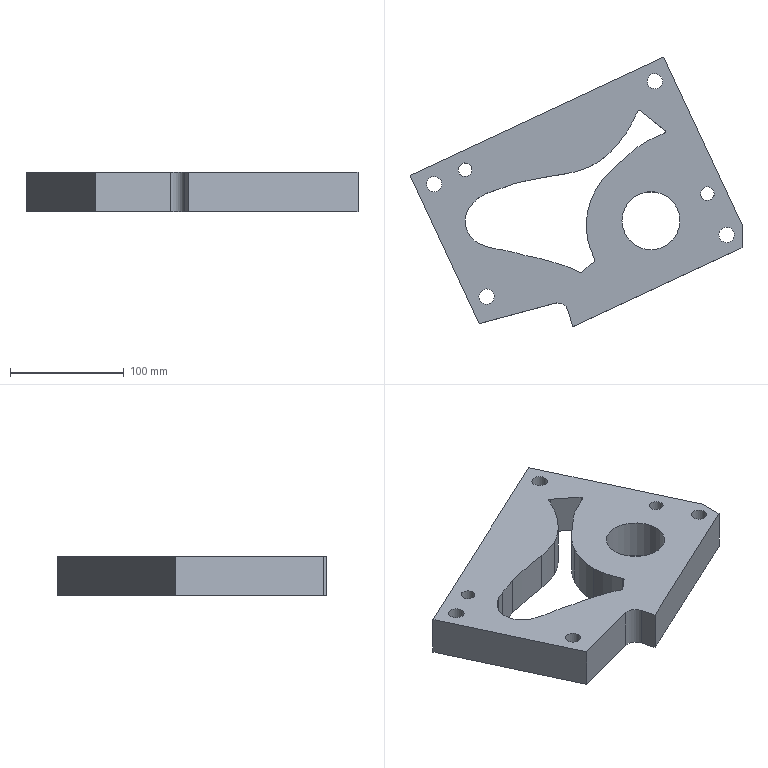Part | NX | features 7 2 | 1 solid | 56 faces | box 291.706 x 237.073 x 35 mm | volume 1073387 mm3 | cylinder 37 | plane 19 | commonest cylinder face diameters 20 x5 3 x4 13.5 x4 12.001 x2 14.11 x2 40.451 x1